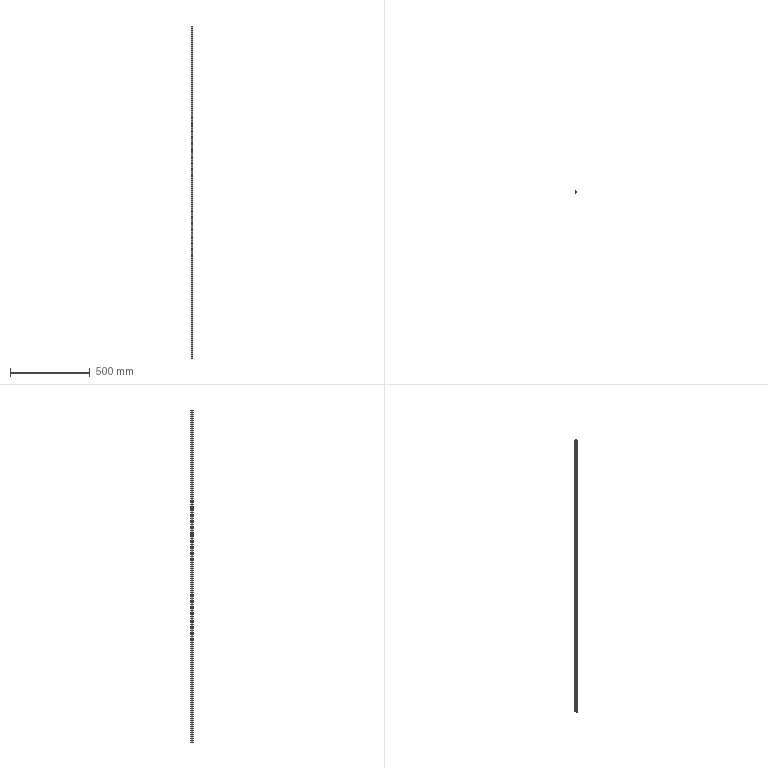Part | SolidWorks | features BaseBody 1, MoveFace 1 | 1 solid | 20 faces | box 10.8 x 17.5 x 2084 mm | volume 164220 mm3 | cylinder 11 | plane 9 | commonest cylinder face diameters 1.6 x2 14 x2 0.4 x1 0.6 x1 0.8 x1 2.6 x1
STEP:
#1=CARTESIAN_POINT('',(-3.236,-11.055,1984.));
#2=VERTEX_POINT('',#1);
#3=CARTESIAN_POINT('',(-4.3,-10.3,1984.));
#4=VERTEX_POINT('',#3);
#5=CARTESIAN_POINT('',(-3.5,-10.3,1984.));
#6=DIRECTION('',(0.,0.,-1.));
#7=DIRECTION('',(1.,0.,0.));
#8=AXIS2_PLACEMENT_3D('',#5,#6,#7);
#9=CIRCLE('',#8,0.8);
#10=EDGE_CURVE('',#2,#4,#9,.T.);
#11=ORIENTED_EDGE('',*,*,#10,.T.);
#12=CARTESIAN_POINT('',(-4.3,-10.3,-100.));
#13=VERTEX_POINT('',#12);
#14=CARTESIAN_POINT('',(-4.3,-10.3,-100.));
#15=DIRECTION('',(0.,0.,-1.));
#16=VECTOR('',#15,1000.);
#17=LINE('',#14,#16);
#18=EDGE_CURVE('',#4,#13,#17,.T.);
#19=ORIENTED_EDGE('',*,*,#18,.T.);
#20=CARTESIAN_POINT('',(-3.236,-11.055,-100.));
#21=VERTEX_POINT('',#20);
#22=CARTESIAN_POINT('',(-3.5,-10.3,-100.));
#23=DIRECTION('',(0.,0.,1.));
#24=DIRECTION('',(-1.,0.,0.));
#25=AXIS2_PLACEMENT_3D('',#22,#23,#24);
#26=CIRCLE('',#25,0.8);
#27=EDGE_CURVE('',#13,#21,#26,.T.);
#28=ORIENTED_EDGE('',*,*,#27,.T.);
#29=CARTESIAN_POINT('',(-3.236,-11.055,-100.));
#30=DIRECTION('',(0.,0.,-1.));
#31=VECTOR('',#30,1000.);
#32=LINE('',#29,#31);
#33=EDGE_CURVE('',#2,#21,#32,.T.);
#34=ORIENTED_EDGE('',*,*,#33,.F.);
#35=EDGE_LOOP('',(#11,#19,#28,#34));
#36=FACE_OUTER_BOUND('',#35,.T.);
#37=CARTESIAN_POINT('',(-3.5,-10.3,-100.));
#38=DIRECTION('',(0.,0.,-1.));
#39=DIRECTION('',(-1.,0.,0.));
#40=AXIS2_PLACEMENT_3D('',#37,#38,#39);
#41=CYLINDRICAL_SURFACE('',#40,0.8);
#42=ADVANCED_FACE('',(#36),#41,.T.);
#43=CARTESIAN_POINT('',(1.184,-6.397,-100.));
#44=VERTEX_POINT('',#43);
#45=CARTESIAN_POINT('',(-5.702,-4.29,-100.));
#46=DIRECTION('',(0.,0.,1.));
#47=DIRECTION('',(-1.,0.,0.));
#48=AXIS2_PLACEMENT_3D('',#45,#46,#47);
#49=CIRCLE('',#48,7.201);
#50=EDGE_CURVE('',#21,#44,#49,.T.);
#51=ORIENTED_EDGE('',*,*,#50,.T.);
#52=CARTESIAN_POINT('',(1.184,-6.397,1984.));
#53=VERTEX_POINT('',#52);
#54=CARTESIAN_POINT('',(1.184,-6.397,-100.));
#55=DIRECTION('',(0.,0.,1.));
#56=VECTOR('',#55,1000.);
#57=LINE('',#54,#56);
#58=EDGE_CURVE('',#44,#53,#57,.T.);
#59=ORIENTED_EDGE('',*,*,#58,.T.);
#60=CARTESIAN_POINT('',(-5.702,-4.29,1984.));
#61=DIRECTION('',(0.,0.,-1.));
#62=DIRECTION('',(1.,0.,0.));
#63=AXIS2_PLACEMENT_3D('',#60,#61,#62);
#64=CIRCLE('',#63,7.201);
#65=EDGE_CURVE('',#53,#2,#64,.T.);
#66=ORIENTED_EDGE('',*,*,#65,.T.);
#67=ORIENTED_EDGE('',*,*,#33,.T.);
#68=EDGE_LOOP('',(#51,#59,#66,#67));
#69=FACE_OUTER_BOUND('',#68,.T.);
#70=CARTESIAN_POINT('',(-5.702,-4.29,-100.));
#71=DIRECTION('',(0.,0.,-1.));
#72=DIRECTION('',(-1.,0.,0.));
#73=AXIS2_PLACEMENT_3D('',#70,#71,#72);
#74=CYLINDRICAL_SURFACE('',#73,7.201);
#75=ADVANCED_FACE('',(#69),#74,.T.);
#76=CARTESIAN_POINT('',(0.9,-6.,-100.));
#77=VERTEX_POINT('',#76);
#78=CARTESIAN_POINT('',(0.9,-6.3,-100.));
#79=DIRECTION('',(0.,0.,1.));
#80=DIRECTION('',(-1.,0.,0.));
#81=AXIS2_PLACEMENT_3D('',#78,#79,#80);
#82=CIRCLE('',#81,0.3);
#83=EDGE_CURVE('',#44,#77,#82,.T.);
#84=ORIENTED_EDGE('',*,*,#83,.T.);
#85=CARTESIAN_POINT('',(0.9,-6.,1984.));
#86=VERTEX_POINT('',#85);
#87=CARTESIAN_POINT('',(0.9,-6.,-100.));
#88=DIRECTION('',(0.,0.,1.));
#89=VECTOR('',#88,1000.);
#90=LINE('',#87,#89);
#91=EDGE_CURVE('',#77,#86,#90,.T.);
#92=ORIENTED_EDGE('',*,*,#91,.T.);
#93=CARTESIAN_POINT('',(0.9,-6.3,1984.));
#94=DIRECTION('',(0.,0.,-1.));
#95=DIRECTION('',(1.,0.,0.));
#96=AXIS2_PLACEMENT_3D('',#93,#94,#95);
#97=CIRCLE('',#96,0.3);
#98=EDGE_CURVE('',#86,#53,#97,.T.);
#99=ORIENTED_EDGE('',*,*,#98,.T.);
#100=ORIENTED_EDGE('',*,*,#58,.F.);
#101=EDGE_LOOP('',(#84,#92,#99,#100));
#102=FACE_OUTER_BOUND('',#101,.T.);
#103=CARTESIAN_POINT('',(0.9,-6.3,-100.));
#104=DIRECTION('',(0.,0.,-1.));
#105=DIRECTION('',(-1.,0.,0.));
#106=AXIS2_PLACEMENT_3D('',#103,#104,#105);
#107=CYLINDRICAL_SURFACE('',#106,0.3);
#108=ADVANCED_FACE('',(#102),#107,.T.);
#109=CARTESIAN_POINT('',(-2.5,-0.5,-100.));
#110=VERTEX_POINT('',#109);
#111=CARTESIAN_POINT('',(-2.5,-6.153,-100.));
#112=VERTEX_POINT('',#111);
#113=CARTESIAN_POINT('',(-2.5,-6.397,-100.));
#114=DIRECTION('',(0.,-1.,0.));
#115=VECTOR('',#114,1000.);
#116=LINE('',#113,#115);
#117=EDGE_CURVE('',#110,#112,#116,.T.);
#118=ORIENTED_EDGE('',*,*,#117,.F.);
#119=CARTESIAN_POINT('',(-4.2,1.695,-100.));
#120=VERTEX_POINT('',#119);
#121=CARTESIAN_POINT('',(-1.701,1.875,-100.));
#122=DIRECTION('',(0.,0.,1.));
#123=DIRECTION('',(-1.,0.,0.));
#124=AXIS2_PLACEMENT_3D('',#121,#122,#123);
#125=CIRCLE('',#124,2.506);
#126=EDGE_CURVE('',#120,#110,#125,.T.);
#127=ORIENTED_EDGE('',*,*,#126,.F.);
#128=CARTESIAN_POINT('',(-4.2,5.1,-100.));
#129=VERTEX_POINT('',#128);
#130=CARTESIAN_POINT('',(-4.2,-6.397,-100.));
#131=DIRECTION('',(0.,-1.,0.));
#132=VECTOR('',#131,1000.);
#133=LINE('',#130,#132);
#134=EDGE_CURVE('',#129,#120,#133,.T.);
#135=ORIENTED_EDGE('',*,*,#134,.F.);
#136=CARTESIAN_POINT('',(-2.892,6.4,-100.));
#137=VERTEX_POINT('',#136);
#138=CARTESIAN_POINT('',(-2.9,5.1,-100.));
#139=DIRECTION('',(0.,0.,1.));
#140=DIRECTION('',(-1.,0.,0.));
#141=AXIS2_PLACEMENT_3D('',#138,#139,#140);
#142=CIRCLE('',#141,1.3);
#143=EDGE_CURVE('',#137,#129,#142,.T.);
#144=ORIENTED_EDGE('',*,*,#143,.F.);
#145=CARTESIAN_POINT('',(0.5,5.5,-100.));
#146=VERTEX_POINT('',#145);
#147=CARTESIAN_POINT('',(-2.934,-0.5999,-100.));
#148=DIRECTION('',(0.,0.,1.));
#149=DIRECTION('',(-1.,0.,0.));
#150=AXIS2_PLACEMENT_3D('',#147,#148,#149);
#151=CIRCLE('',#150,7.);
#152=EDGE_CURVE('',#146,#137,#151,.T.);
#153=ORIENTED_EDGE('',*,*,#152,.F.);
#154=CARTESIAN_POINT('',(5.5,1.7,-100.));
#155=VERTEX_POINT('',#154);
#156=CARTESIAN_POINT('',(5.5,1.7,-100.));
#157=DIRECTION('',(-0.7962,0.6051,0.));
#158=VECTOR('',#157,1000.);
#159=LINE('',#156,#158);
#160=EDGE_CURVE('',#155,#146,#159,.T.);
#161=ORIENTED_EDGE('',*,*,#160,.F.);
#162=CARTESIAN_POINT('',(6.458,-0.2215,-100.));
#163=VERTEX_POINT('',#162);
#164=CARTESIAN_POINT('',(6.458,-0.2215,-100.));
#165=DIRECTION('',(-0.4462,0.8949,0.));
#166=VECTOR('',#165,1000.);
#167=LINE('',#164,#166);
#168=EDGE_CURVE('',#163,#155,#167,.T.);
#169=ORIENTED_EDGE('',*,*,#168,.F.);
#170=CARTESIAN_POINT('',(5.895,-0.7433,-100.));
#171=VERTEX_POINT('',#170);
#172=CARTESIAN_POINT('',(6.1,-0.4,-100.));
#173=DIRECTION('',(0.,0.,1.));
#174=DIRECTION('',(-1.,0.,0.));
#175=AXIS2_PLACEMENT_3D('',#172,#173,#174);
#176=CIRCLE('',#175,0.4);
#177=EDGE_CURVE('',#171,#163,#176,.T.);
#178=ORIENTED_EDGE('',*,*,#177,.F.);
#179=CARTESIAN_POINT('',(3.,0.,-100.));
#180=VERTEX_POINT('',#179);
#181=CARTESIAN_POINT('',(2.746,-6.995,-100.));
#182=DIRECTION('',(0.,0.,-1.));
#183=DIRECTION('',(-1.,0.,0.));
#184=AXIS2_PLACEMENT_3D('',#181,#182,#183);
#185=CIRCLE('',#184,7.);
#186=EDGE_CURVE('',#180,#171,#185,.T.);
#187=ORIENTED_EDGE('',*,*,#186,.F.);
#188=CARTESIAN_POINT('',(0.,0.,-100.));
#189=VERTEX_POINT('',#188);
#190=CARTESIAN_POINT('',(-6.814,0.,-100.));
#191=DIRECTION('',(1.,0.,0.));
#192=VECTOR('',#191,1000.);
#193=LINE('',#190,#192);
#194=EDGE_CURVE('',#189,#180,#193,.T.);
#195=ORIENTED_EDGE('',*,*,#194,.F.);
#196=CARTESIAN_POINT('',(0.,-5.8,-100.));
#197=VERTEX_POINT('',#196);
#198=CARTESIAN_POINT('',(0.,-6.397,-100.));
#199=DIRECTION('',(0.,1.,0.));
#200=VECTOR('',#199,1000.);
#201=LINE('',#198,#200);
#202=EDGE_CURVE('',#197,#189,#201,.T.);
#203=ORIENTED_EDGE('',*,*,#202,.F.);
#204=CARTESIAN_POINT('',(0.2,-6.,-100.));
#205=VERTEX_POINT('',#204);
#206=CARTESIAN_POINT('',(0.2,-5.8,-100.));
#207=DIRECTION('',(0.,0.,1.));
#208=DIRECTION('',(-1.,0.,0.));
#209=AXIS2_PLACEMENT_3D('',#206,#207,#208);
#210=CIRCLE('',#209,0.2);
#211=EDGE_CURVE('',#197,#205,#210,.T.);
#212=ORIENTED_EDGE('',*,*,#211,.T.);
#213=CARTESIAN_POINT('',(-6.814,-6.,-100.));
#214=DIRECTION('',(-1.,0.,0.));
#215=VECTOR('',#214,1000.);
#216=LINE('',#213,#215);
#217=EDGE_CURVE('',#77,#205,#216,.T.);
#218=ORIENTED_EDGE('',*,*,#217,.F.);
#219=ORIENTED_EDGE('',*,*,#83,.F.);
#220=ORIENTED_EDGE('',*,*,#50,.F.);
#221=ORIENTED_EDGE('',*,*,#27,.F.);
#222=CARTESIAN_POINT('',(-3.998,-9.674,-100.));
#223=VERTEX_POINT('',#222);
#224=CARTESIAN_POINT('',(-3.5,-10.3,-100.));
#225=DIRECTION('',(0.,0.,1.));
#226=DIRECTION('',(-1.,0.,0.));
#227=AXIS2_PLACEMENT_3D('',#224,#225,#226);
#228=CIRCLE('',#227,0.8);
#229=EDGE_CURVE('',#223,#13,#228,.T.);
#230=ORIENTED_EDGE('',*,*,#229,.F.);
#231=CARTESIAN_POINT('',(-6.814,-6.397,-100.));
#232=DIRECTION('',(0.,0.,-1.));
#233=DIRECTION('',(-1.,0.,0.));
#234=AXIS2_PLACEMENT_3D('',#231,#232,#233);
#235=CIRCLE('',#234,4.321);
#236=EDGE_CURVE('',#112,#223,#235,.T.);
#237=ORIENTED_EDGE('',*,*,#236,.F.);
#238=EDGE_LOOP('',(#118,#127,#135,#144,#153,#161,#169,#178,#187,#195,#203,#212,#218,#219,#220,#221,#230,#237));
#239=FACE_OUTER_BOUND('',#238,.T.);
#240=CARTESIAN_POINT('',(-6.814,-6.397,-100.));
#241=DIRECTION('',(0.,0.,1.));
#242=DIRECTION('',(1.,0.,0.));
#243=AXIS2_PLACEMENT_3D('',#240,#241,#242);
#244=PLANE('',#243);
#245=ADVANCED_FACE('',(#239),#244,.F.);
#246=ORIENTED_EDGE('',*,*,#18,.F.);
#247=CARTESIAN_POINT('',(-3.998,-9.674,1984.));
#248=VERTEX_POINT('',#247);
#249=CARTESIAN_POINT('',(-3.5,-10.3,1984.));
#250=DIRECTION('',(0.,0.,-1.));
#251=DIRECTION('',(1.,0.,0.));
#252=AXIS2_PLACEMENT_3D('',#249,#250,#251);
#253=CIRCLE('',#252,0.8);
#254=EDGE_CURVE('',#4,#248,#253,.T.);
#255=ORIENTED_EDGE('',*,*,#254,.T.);
#256=CARTESIAN_POINT('',(-3.998,-9.674,-100.));
#257=DIRECTION('',(0.,0.,-1.));
#258=VECTOR('',#257,1000.);
#259=LINE('',#256,#258);
#260=EDGE_CURVE('',#248,#223,#259,.T.);
#261=ORIENTED_EDGE('',*,*,#260,.T.);
#262=ORIENTED_EDGE('',*,*,#229,.T.);
#263=EDGE_LOOP('',(#246,#255,#261,#262));
#264=FACE_OUTER_BOUND('',#263,.T.);
#265=CARTESIAN_POINT('',(-3.5,-10.3,-100.));
#266=DIRECTION('',(0.,0.,-1.));
#267=DIRECTION('',(-1.,0.,0.));
#268=AXIS2_PLACEMENT_3D('',#265,#266,#267);
#269=CYLINDRICAL_SURFACE('',#268,0.8);
#270=ADVANCED_FACE('',(#264),#269,.T.);
#271=CARTESIAN_POINT('',(-4.2,1.695,1984.));
#272=VERTEX_POINT('',#271);
#273=CARTESIAN_POINT('',(-2.5,-0.5,1984.));
#274=VERTEX_POINT('',#273);
#275=CARTESIAN_POINT('',(-1.701,1.875,1984.));
#276=DIRECTION('',(0.,0.,1.));
#277=DIRECTION('',(1.,0.,0.));
#278=AXIS2_PLACEMENT_3D('',#275,#276,#277);
#279=CIRCLE('',#278,2.506);
#280=EDGE_CURVE('',#272,#274,#279,.T.);
#281=ORIENTED_EDGE('',*,*,#280,.T.);
#282=CARTESIAN_POINT('',(-2.5,-6.153,1984.));
#283=VERTEX_POINT('',#282);
#284=CARTESIAN_POINT('',(-2.5,-6.397,1984.));
#285=DIRECTION('',(0.,-1.,0.));
#286=VECTOR('',#285,1000.);
#287=LINE('',#284,#286);
#288=EDGE_CURVE('',#274,#283,#287,.T.);
#289=ORIENTED_EDGE('',*,*,#288,.T.);
#290=CARTESIAN_POINT('',(-6.814,-6.397,1984.));
#291=DIRECTION('',(0.,0.,-1.));
#292=DIRECTION('',(1.,0.,0.));
#293=AXIS2_PLACEMENT_3D('',#290,#291,#292);
#294=CIRCLE('',#293,4.321);
#295=EDGE_CURVE('',#283,#248,#294,.T.);
#296=ORIENTED_EDGE('',*,*,#295,.T.);
#297=ORIENTED_EDGE('',*,*,#254,.F.);
#298=ORIENTED_EDGE('',*,*,#10,.F.);
#299=ORIENTED_EDGE('',*,*,#65,.F.);
#300=ORIENTED_EDGE('',*,*,#98,.F.);
#301=CARTESIAN_POINT('',(0.2,-6.,1984.));
#302=VERTEX_POINT('',#301);
#303=CARTESIAN_POINT('',(-6.814,-6.,1984.));
#304=DIRECTION('',(-1.,0.,0.));
#305=VECTOR('',#304,1000.);
#306=LINE('',#303,#305);
#307=EDGE_CURVE('',#86,#302,#306,.T.);
#308=ORIENTED_EDGE('',*,*,#307,.T.);
#309=CARTESIAN_POINT('',(0.,-5.8,1984.));
#310=VERTEX_POINT('',#309);
#311=CARTESIAN_POINT('',(0.2,-5.8,1984.));
#312=DIRECTION('',(0.,0.,-1.));
#313=DIRECTION('',(1.,0.,0.));
#314=AXIS2_PLACEMENT_3D('',#311,#312,#313);
#315=CIRCLE('',#314,0.2);
#316=EDGE_CURVE('',#302,#310,#315,.T.);
#317=ORIENTED_EDGE('',*,*,#316,.T.);
#318=CARTESIAN_POINT('',(0.,0.,1984.));
#319=VERTEX_POINT('',#318);
#320=CARTESIAN_POINT('',(0.,-6.397,1984.));
#321=DIRECTION('',(0.,1.,0.));
#322=VECTOR('',#321,1000.);
#323=LINE('',#320,#322);
#324=EDGE_CURVE('',#310,#319,#323,.T.);
#325=ORIENTED_EDGE('',*,*,#324,.T.);
#326=CARTESIAN_POINT('',(3.,0.,1984.));
#327=VERTEX_POINT('',#326);
#328=CARTESIAN_POINT('',(-6.814,0.,1984.));
#329=DIRECTION('',(1.,0.,0.));
#330=VECTOR('',#329,1000.);
#331=LINE('',#328,#330);
#332=EDGE_CURVE('',#319,#327,#331,.T.);
#333=ORIENTED_EDGE('',*,*,#332,.T.);
#334=CARTESIAN_POINT('',(5.895,-0.7433,1984.));
#335=VERTEX_POINT('',#334);
#336=CARTESIAN_POINT('',(2.746,-6.995,1984.));
#337=DIRECTION('',(0.,0.,-1.));
#338=DIRECTION('',(1.,0.,0.));
#339=AXIS2_PLACEMENT_3D('',#336,#337,#338);
#340=CIRCLE('',#339,7.);
#341=EDGE_CURVE('',#327,#335,#340,.T.);
#342=ORIENTED_EDGE('',*,*,#341,.T.);
#343=CARTESIAN_POINT('',(6.458,-0.2215,1984.));
#344=VERTEX_POINT('',#343);
#345=CARTESIAN_POINT('',(6.1,-0.4,1984.));
#346=DIRECTION('',(0.,0.,-1.));
#347=DIRECTION('',(1.,0.,0.));
#348=AXIS2_PLACEMENT_3D('',#345,#346,#347);
#349=CIRCLE('',#348,0.4);
#350=EDGE_CURVE('',#344,#335,#349,.T.);
#351=ORIENTED_EDGE('',*,*,#350,.F.);
#352=CARTESIAN_POINT('',(5.5,1.7,1984.));
#353=VERTEX_POINT('',#352);
#354=CARTESIAN_POINT('',(6.282,0.1323,1984.));
#355=DIRECTION('',(-0.4462,0.8949,0.));
#356=VECTOR('',#355,1000.);
#357=LINE('',#354,#356);
#358=EDGE_CURVE('',#344,#353,#357,.T.);
#359=ORIENTED_EDGE('',*,*,#358,.T.);
#360=CARTESIAN_POINT('',(0.5,5.5,1984.));
#361=VERTEX_POINT('',#360);
#362=CARTESIAN_POINT('',(1.595,4.668,1984.));
#363=DIRECTION('',(-0.7962,0.6051,0.));
#364=VECTOR('',#363,1000.);
#365=LINE('',#362,#364);
#366=EDGE_CURVE('',#353,#361,#365,.T.);
#367=ORIENTED_EDGE('',*,*,#366,.T.);
#368=CARTESIAN_POINT('',(-2.892,6.4,1984.));
#369=VERTEX_POINT('',#368);
#370=CARTESIAN_POINT('',(-2.934,-0.5999,1984.));
#371=DIRECTION('',(0.,0.,1.));
#372=DIRECTION('',(1.,0.,0.));
#373=AXIS2_PLACEMENT_3D('',#370,#371,#372);
#374=CIRCLE('',#373,7.);
#375=EDGE_CURVE('',#361,#369,#374,.T.);
#376=ORIENTED_EDGE('',*,*,#375,.T.);
#377=CARTESIAN_POINT('',(-4.2,5.1,1984.));
#378=VERTEX_POINT('',#377);
#379=CARTESIAN_POINT('',(-2.9,5.1,1984.));
#380=DIRECTION('',(0.,0.,1.));
#381=DIRECTION('',(1.,0.,0.));
#382=AXIS2_PLACEMENT_3D('',#379,#380,#381);
#383=CIRCLE('',#382,1.3);
#384=EDGE_CURVE('',#369,#378,#383,.T.);
#385=ORIENTED_EDGE('',*,*,#384,.T.);
#386=CARTESIAN_POINT('',(-4.2,-6.397,1984.));
#387=DIRECTION('',(0.,-1.,0.));
#388=VECTOR('',#387,1000.);
#389=LINE('',#386,#388);
#390=EDGE_CURVE('',#378,#272,#389,.T.);
#391=ORIENTED_EDGE('',*,*,#390,.T.);
#392=EDGE_LOOP('',(#281,#289,#296,#297,#298,#299,#300,#308,#317,#325,#333,#342,#351,#359,#367,#376,#385,#391));
#393=FACE_OUTER_BOUND('',#392,.T.);
#394=CARTESIAN_POINT('',(-6.814,-6.397,1984.));
#395=DIRECTION('',(0.,0.,1.));
#396=DIRECTION('',(1.,0.,0.));
#397=AXIS2_PLACEMENT_3D('',#394,#395,#396);
#398=PLANE('',#397);
#399=ADVANCED_FACE('',(#393),#398,.T.);
#400=ORIENTED_EDGE('',*,*,#217,.T.);
#401=CARTESIAN_POINT('',(0.2,-6.,-100.));
#402=DIRECTION('',(0.,0.,1.));
#403=VECTOR('',#402,1000.);
#404=LINE('',#401,#403);
#405=EDGE_CURVE('',#205,#302,#404,.T.);
#406=ORIENTED_EDGE('',*,*,#405,.T.);
#407=ORIENTED_EDGE('',*,*,#307,.F.);
#408=ORIENTED_EDGE('',*,*,#91,.F.);
#409=EDGE_LOOP('',(#400,#406,#407,#408));
#410=FACE_OUTER_BOUND('',#409,.T.);
#411=CARTESIAN_POINT('',(0.9,-6.,-100.));
#412=DIRECTION('',(0.,1.,0.));
#413=DIRECTION('',(0.,0.,1.));
#414=AXIS2_PLACEMENT_3D('',#411,#412,#413);
#415=PLANE('',#414);
#416=ADVANCED_FACE('',(#410),#415,.T.);
#417=CARTESIAN_POINT('',(-2.5,-6.153,-100.));
#418=DIRECTION('',(0.,0.,1.));
#419=VECTOR('',#418,1000.);
#420=LINE('',#417,#419);
#421=EDGE_CURVE('',#112,#283,#420,.T.);
#422=ORIENTED_EDGE('',*,*,#421,.F.);
#423=ORIENTED_EDGE('',*,*,#236,.T.);
#424=ORIENTED_EDGE('',*,*,#260,.F.);
#425=ORIENTED_EDGE('',*,*,#295,.F.);
#426=EDGE_LOOP('',(#422,#423,#424,#425));
#427=FACE_OUTER_BOUND('',#426,.T.);
#428=CARTESIAN_POINT('',(-6.814,-6.397,-100.));
#429=DIRECTION('',(0.,0.,-1.));
#430=DIRECTION('',(-1.,0.,0.));
#431=AXIS2_PLACEMENT_3D('',#428,#429,#430);
#432=CYLINDRICAL_SURFACE('',#431,4.321);
#433=ADVANCED_FACE('',(#427),#432,.F.);
#434=ORIENTED_EDGE('',*,*,#117,.T.);
#435=ORIENTED_EDGE('',*,*,#421,.T.);
#436=ORIENTED_EDGE('',*,*,#288,.F.);
#437=CARTESIAN_POINT('',(-2.5,-0.5,-100.));
#438=DIRECTION('',(0.,0.,-1.));
#439=VECTOR('',#438,1000.);
#440=LINE('',#437,#439);
#441=EDGE_CURVE('',#274,#110,#440,.T.);
#442=ORIENTED_EDGE('',*,*,#441,.T.);
#443=EDGE_LOOP('',(#434,#435,#436,#442));
#444=FACE_OUTER_BOUND('',#443,.T.);
#445=CARTESIAN_POINT('',(-2.5,-0.5,-100.));
#446=DIRECTION('',(-1.,0.,0.));
#447=DIRECTION('',(0.,0.,1.));
#448=AXIS2_PLACEMENT_3D('',#445,#446,#447);
#449=PLANE('',#448);
#450=ADVANCED_FACE('',(#444),#449,.T.);
#451=ORIENTED_EDGE('',*,*,#126,.T.);
#452=ORIENTED_EDGE('',*,*,#441,.F.);
#453=ORIENTED_EDGE('',*,*,#280,.F.);
#454=CARTESIAN_POINT('',(-4.2,1.695,-100.));
#455=DIRECTION('',(0.,0.,-1.));
#456=VECTOR('',#455,1000.);
#457=LINE('',#454,#456);
#458=EDGE_CURVE('',#272,#120,#457,.T.);
#459=ORIENTED_EDGE('',*,*,#458,.T.);
#460=EDGE_LOOP('',(#451,#452,#453,#459));
#461=FACE_OUTER_BOUND('',#460,.T.);
#462=CARTESIAN_POINT('',(-1.701,1.875,-100.));
#463=DIRECTION('',(0.,0.,-1.));
#464=DIRECTION('',(-1.,0.,0.));
#465=AXIS2_PLACEMENT_3D('',#462,#463,#464);
#466=CYLINDRICAL_SURFACE('',#465,2.506);
#467=ADVANCED_FACE('',(#461),#466,.T.);
#468=ORIENTED_EDGE('',*,*,#134,.T.);
#469=ORIENTED_EDGE('',*,*,#458,.F.);
#470=ORIENTED_EDGE('',*,*,#390,.F.);
#471=CARTESIAN_POINT('',(-4.2,5.1,-100.));
#472=DIRECTION('',(0.,0.,-1.));
#473=VECTOR('',#472,1000.);
#474=LINE('',#471,#473);
#475=EDGE_CURVE('',#378,#129,#474,.T.);
#476=ORIENTED_EDGE('',*,*,#475,.T.);
#477=EDGE_LOOP('',(#468,#469,#470,#476));
#478=FACE_OUTER_BOUND('',#477,.T.);
#479=CARTESIAN_POINT('',(-4.2,5.1,-100.));
#480=DIRECTION('',(-1.,0.,0.));
#481=DIRECTION('',(0.,0.,1.));
#482=AXIS2_PLACEMENT_3D('',#479,#480,#481);
#483=PLANE('',#482);
#484=ADVANCED_FACE('',(#478),#483,.T.);
#485=ORIENTED_EDGE('',*,*,#143,.T.);
#486=ORIENTED_EDGE('',*,*,#475,.F.);
#487=ORIENTED_EDGE('',*,*,#384,.F.);
#488=CARTESIAN_POINT('',(-2.892,6.4,-100.));
#489=DIRECTION('',(0.,0.,-1.));
#490=VECTOR('',#489,1000.);
#491=LINE('',#488,#490);
#492=EDGE_CURVE('',#369,#137,#491,.T.);
#493=ORIENTED_EDGE('',*,*,#492,.T.);
#494=EDGE_LOOP('',(#485,#486,#487,#493));
#495=FACE_OUTER_BOUND('',#494,.T.);
#496=CARTESIAN_POINT('',(-2.9,5.1,-100.));
#497=DIRECTION('',(0.,0.,-1.));
#498=DIRECTION('',(-1.,0.,0.));
#499=AXIS2_PLACEMENT_3D('',#496,#497,#498);
#500=CYLINDRICAL_SURFACE('',#499,1.3);
#501=ADVANCED_FACE('',(#495),#500,.T.);
#502=ORIENTED_EDGE('',*,*,#152,.T.);
#503=ORIENTED_EDGE('',*,*,#492,.F.);
#504=ORIENTED_EDGE('',*,*,#375,.F.);
#505=CARTESIAN_POINT('',(0.5,5.5,-100.));
#506=DIRECTION('',(0.,0.,-1.));
#507=VECTOR('',#506,1000.);
#508=LINE('',#505,#507);
#509=EDGE_CURVE('',#361,#146,#508,.T.);
#510=ORIENTED_EDGE('',*,*,#509,.T.);
#511=EDGE_LOOP('',(#502,#503,#504,#510));
#512=FACE_OUTER_BOUND('',#511,.T.);
#513=CARTESIAN_POINT('',(-2.934,-0.5999,-100.));
#514=DIRECTION('',(0.,0.,-1.));
#515=DIRECTION('',(-1.,0.,0.));
#516=AXIS2_PLACEMENT_3D('',#513,#514,#515);
#517=CYLINDRICAL_SURFACE('',#516,7.);
#518=ADVANCED_FACE('',(#512),#517,.T.);
#519=ORIENTED_EDGE('',*,*,#160,.T.);
#520=ORIENTED_EDGE('',*,*,#509,.F.);
#521=ORIENTED_EDGE('',*,*,#366,.F.);
#522=CARTESIAN_POINT('',(5.5,1.7,-100.));
#523=DIRECTION('',(0.,0.,-1.));
#524=VECTOR('',#523,1000.);
#525=LINE('',#522,#524);
#526=EDGE_CURVE('',#353,#155,#525,.T.);
#527=ORIENTED_EDGE('',*,*,#526,.T.);
#528=EDGE_LOOP('',(#519,#520,#521,#527));
#529=FACE_OUTER_BOUND('',#528,.T.);
#530=CARTESIAN_POINT('',(5.5,1.7,-100.));
#531=DIRECTION('',(0.6051,0.7962,0.));
#532=DIRECTION('',(-0.7962,0.6051,0.));
#533=AXIS2_PLACEMENT_3D('',#530,#531,#532);
#534=PLANE('',#533);
#535=ADVANCED_FACE('',(#529),#534,.T.);
#536=ORIENTED_EDGE('',*,*,#168,.T.);
#537=ORIENTED_EDGE('',*,*,#526,.F.);
#538=ORIENTED_EDGE('',*,*,#358,.F.);
#539=CARTESIAN_POINT('',(6.458,-0.2215,-100.));
#540=DIRECTION('',(0.,0.,-1.));
#541=VECTOR('',#540,1000.);
#542=LINE('',#539,#541);
#543=EDGE_CURVE('',#344,#163,#542,.T.);
#544=ORIENTED_EDGE('',*,*,#543,.T.);
#545=EDGE_LOOP('',(#536,#537,#538,#544));
#546=FACE_OUTER_BOUND('',#545,.T.);
#547=CARTESIAN_POINT('',(6.458,-0.2215,-100.));
#548=DIRECTION('',(0.8949,0.4462,0.));
#549=DIRECTION('',(-0.4462,0.8949,0.));
#550=AXIS2_PLACEMENT_3D('',#547,#548,#549);
#551=PLANE('',#550);
#552=ADVANCED_FACE('',(#546),#551,.T.);
#553=CARTESIAN_POINT('',(3.,0.,-100.));
#554=DIRECTION('',(0.,0.,1.));
#555=VECTOR('',#554,1000.);
#556=LINE('',#553,#555);
#557=EDGE_CURVE('',#180,#327,#556,.T.);
#558=ORIENTED_EDGE('',*,*,#557,.F.);
#559=ORIENTED_EDGE('',*,*,#186,.T.);
#560=CARTESIAN_POINT('',(5.895,-0.7433,-100.));
#561=DIRECTION('',(0.,0.,-1.));
#562=VECTOR('',#561,1000.);
#563=LINE('',#560,#562);
#564=EDGE_CURVE('',#335,#171,#563,.T.);
#565=ORIENTED_EDGE('',*,*,#564,.F.);
#566=ORIENTED_EDGE('',*,*,#341,.F.);
#567=EDGE_LOOP('',(#558,#559,#565,#566));
#568=FACE_OUTER_BOUND('',#567,.T.);
#569=CARTESIAN_POINT('',(2.746,-6.995,-100.));
#570=DIRECTION('',(0.,0.,-1.));
#571=DIRECTION('',(-1.,0.,0.));
#572=AXIS2_PLACEMENT_3D('',#569,#570,#571);
#573=CYLINDRICAL_SURFACE('',#572,7.);
#574=ADVANCED_FACE('',(#568),#573,.F.);
#575=ORIENTED_EDGE('',*,*,#194,.T.);
#576=ORIENTED_EDGE('',*,*,#557,.T.);
#577=ORIENTED_EDGE('',*,*,#332,.F.);
#578=CARTESIAN_POINT('',(0.,0.,-100.));
#579=DIRECTION('',(0.,0.,-1.));
#580=VECTOR('',#579,1000.);
#581=LINE('',#578,#580);
#582=EDGE_CURVE('',#319,#189,#581,.T.);
#583=ORIENTED_EDGE('',*,*,#582,.T.);
#584=EDGE_LOOP('',(#575,#576,#577,#583));
#585=FACE_OUTER_BOUND('',#584,.T.);
#586=CARTESIAN_POINT('',(0.,0.,-100.));
#587=DIRECTION('',(0.,-1.,0.));
#588=DIRECTION('',(0.,0.,-1.));
#589=AXIS2_PLACEMENT_3D('',#586,#587,#588);
#590=PLANE('',#589);
#591=ADVANCED_FACE('',(#585),#590,.T.);
#592=ORIENTED_EDGE('',*,*,#202,.T.);
#593=ORIENTED_EDGE('',*,*,#582,.F.);
#594=ORIENTED_EDGE('',*,*,#324,.F.);
#595=CARTESIAN_POINT('',(0.,-5.8,-100.));
#596=DIRECTION('',(0.,0.,-1.));
#597=VECTOR('',#596,1000.);
#598=LINE('',#595,#597);
#599=EDGE_CURVE('',#310,#197,#598,.T.);
#600=ORIENTED_EDGE('',*,*,#599,.T.);
#601=EDGE_LOOP('',(#592,#593,#594,#600));
#602=FACE_OUTER_BOUND('',#601,.T.);
#603=CARTESIAN_POINT('',(0.,-5.8,-100.));
#604=DIRECTION('',(1.,0.,0.));
#605=DIRECTION('',(0.,0.,-1.));
#606=AXIS2_PLACEMENT_3D('',#603,#604,#605);
#607=PLANE('',#606);
#608=ADVANCED_FACE('',(#602),#607,.T.);
#609=ORIENTED_EDGE('',*,*,#405,.F.);
#610=ORIENTED_EDGE('',*,*,#211,.F.);
#611=ORIENTED_EDGE('',*,*,#599,.F.);
#612=ORIENTED_EDGE('',*,*,#316,.F.);
#613=EDGE_LOOP('',(#609,#610,#611,#612));
#614=FACE_OUTER_BOUND('',#613,.T.);
#615=CARTESIAN_POINT('',(0.2,-5.8,-100.));
#616=DIRECTION('',(0.,0.,-1.));
#617=DIRECTION('',(-1.,0.,0.));
#618=AXIS2_PLACEMENT_3D('',#615,#616,#617);
#619=CYLINDRICAL_SURFACE('',#618,0.2);
#620=ADVANCED_FACE('',(#614),#619,.F.);
#621=ORIENTED_EDGE('',*,*,#177,.T.);
#622=ORIENTED_EDGE('',*,*,#543,.F.);
#623=ORIENTED_EDGE('',*,*,#350,.T.);
#624=ORIENTED_EDGE('',*,*,#564,.T.);
#625=EDGE_LOOP('',(#621,#622,#623,#624));
#626=FACE_OUTER_BOUND('',#625,.T.);
#627=CARTESIAN_POINT('',(6.1,-0.4,-100.));
#628=DIRECTION('',(0.,0.,-1.));
#629=DIRECTION('',(-1.,0.,0.));
#630=AXIS2_PLACEMENT_3D('',#627,#628,#629);
#631=CYLINDRICAL_SURFACE('',#630,0.4);
#632=ADVANCED_FACE('',(#626),#631,.T.);
#633=CLOSED_SHELL('',(#42,#75,#108,#245,#270,#399,#416,#433,#450,#467,#484,#501,#518,#535,#552,#574,#591,#608,#620,#632));
#634=MANIFOLD_SOLID_BREP('',#633);
#635=CARTESIAN_POINT('',(0.,0.,0.));
#636=DIRECTION('',(0.,0.,1.));
#637=DIRECTION('',(1.,0.,0.));
#638=AXIS2_PLACEMENT_3D('',#635,#636,#637);
#639=(LENGTH_UNIT()NAMED_UNIT(*)SI_UNIT(.MILLI.,.METRE.));
#640=UNCERTAINTY_MEASURE_WITH_UNIT(LENGTH_MEASURE(0.00001),#639,'','');
#641=(NAMED_UNIT(*)PLANE_ANGLE_UNIT()SI_UNIT($,.RADIAN.));
#642=(NAMED_UNIT(*)SI_UNIT($,.STERADIAN.)SOLID_ANGLE_UNIT());
#643=(GEOMETRIC_REPRESENTATION_CONTEXT(3)GLOBAL_UNCERTAINTY_ASSIGNED_CONTEXT((#640))GLOBAL_UNIT_ASSIGNED_CONTEXT((#639,#641,#642))REPRESENTATION_CONTEXT('',''));
#644=ADVANCED_BREP_SHAPE_REPRESENTATION('',(#634,#638),#643);